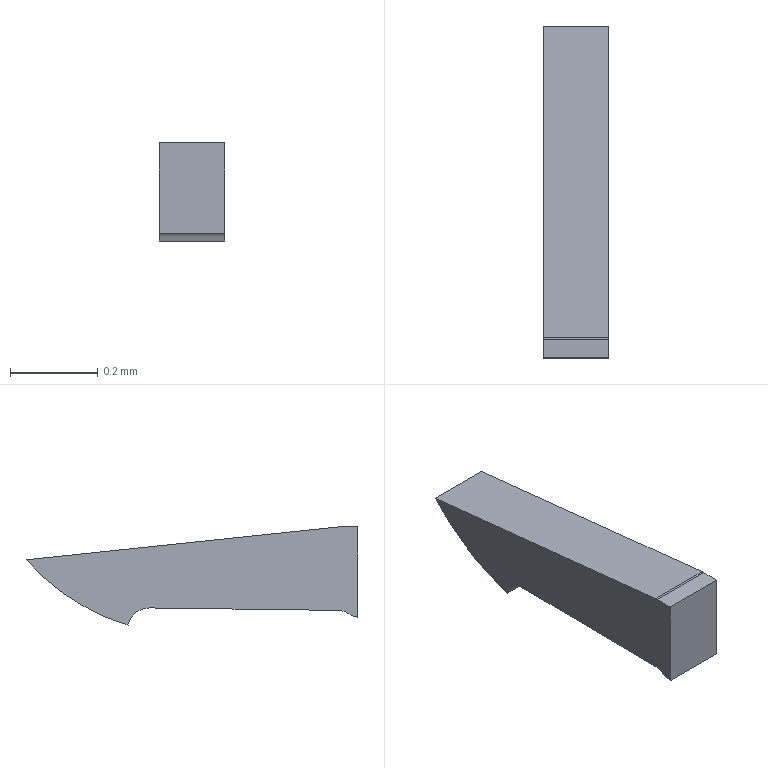Part | Creo | 1 solid | 11 faces | box 0.15 x 0.7581 x 0.2242 mm | volume 0.01667 mm3 | plane 6 | cylinder 5 | commonest cylinder face diameters 0.1 x4 1 x1
STEP:
#1=CARTESIAN_POINT('',(0.,0.,0.));
#2=DIRECTION('',(0.,0.,1.));
#3=DIRECTION('',(1.,0.,0.));
#4=AXIS2_PLACEMENT_3D('',#1,#2,#3);
#5=CARTESIAN_POINT('',(1.21,1.33,-0.16));
#6=VERTEX_POINT('',#5);
#7=CARTESIAN_POINT('',(1.21,1.33,-0.3661));
#8=VERTEX_POINT('',#7);
#9=CARTESIAN_POINT('',(1.21,1.33,-0.16));
#10=DIRECTION('',(0.,0.,-1.));
#11=VECTOR('',#10,0.2061);
#12=LINE('',#9,#11);
#13=EDGE_CURVE('',#6,#8,#12,.T.);
#14=ORIENTED_EDGE('',*,*,#13,.F.);
#15=CARTESIAN_POINT('',(1.21,1.372,-0.16));
#16=VERTEX_POINT('',#15);
#17=CARTESIAN_POINT('',(1.21,1.372,-0.16));
#18=DIRECTION('',(0.,-1.,0.));
#19=VECTOR('',#18,0.04168);
#20=LINE('',#17,#19);
#21=EDGE_CURVE('',#16,#6,#20,.T.);
#22=ORIENTED_EDGE('',*,*,#21,.F.);
#23=CARTESIAN_POINT('',(1.21,1.377,-0.1603));
#24=VERTEX_POINT('',#23);
#25=CARTESIAN_POINT('',(1.21,1.372,-0.21));
#26=DIRECTION('',(-1.,0.,0.));
#27=DIRECTION('',(0.,0.,1.));
#28=AXIS2_PLACEMENT_3D('',#25,#26,#27);
#29=CIRCLE('',#28,0.05);
#30=EDGE_CURVE('',#16,#24,#29,.T.);
#31=ORIENTED_EDGE('',*,*,#30,.T.);
#32=CARTESIAN_POINT('',(1.21,2.088,-0.235));
#33=VERTEX_POINT('',#32);
#34=CARTESIAN_POINT('',(1.21,1.377,-0.1603));
#35=DIRECTION('',(0.,0.9945,-0.1045));
#36=VECTOR('',#35,0.7151);
#37=LINE('',#34,#36);
#38=EDGE_CURVE('',#24,#33,#37,.T.);
#39=ORIENTED_EDGE('',*,*,#38,.T.);
#40=CARTESIAN_POINT('',(1.21,1.855,-0.3842));
#41=VERTEX_POINT('',#40);
#42=CARTESIAN_POINT('',(1.21,1.712,0.09503));
#43=DIRECTION('',(-1.,0.,0.));
#44=DIRECTION('',(0.,0.7512,-0.6601));
#45=AXIS2_PLACEMENT_3D('',#42,#43,#44);
#46=CIRCLE('',#45,0.5);
#47=EDGE_CURVE('',#33,#41,#46,.T.);
#48=ORIENTED_EDGE('',*,*,#47,.T.);
#49=CARTESIAN_POINT('',(1.21,1.806,-0.345));
#50=VERTEX_POINT('',#49);
#51=CARTESIAN_POINT('',(1.21,1.806,-0.395));
#52=DIRECTION('',(1.,0.,0.));
#53=DIRECTION('',(0.,0.9762,0.2167));
#54=AXIS2_PLACEMENT_3D('',#51,#52,#53);
#55=CIRCLE('',#54,0.05);
#56=EDGE_CURVE('',#41,#50,#55,.T.);
#57=ORIENTED_EDGE('',*,*,#56,.T.);
#58=CARTESIAN_POINT('',(1.21,1.377,-0.3506));
#59=VERTEX_POINT('',#58);
#60=CARTESIAN_POINT('',(1.21,1.806,-0.345));
#61=DIRECTION('',(0.,-0.9999,-0.01302));
#62=VECTOR('',#61,0.4289);
#63=LINE('',#60,#62);
#64=EDGE_CURVE('',#50,#59,#63,.T.);
#65=ORIENTED_EDGE('',*,*,#64,.T.);
#66=CARTESIAN_POINT('',(1.21,1.35,-0.3586));
#67=VERTEX_POINT('',#66);
#68=CARTESIAN_POINT('',(1.21,1.378,-0.4006));
#69=DIRECTION('',(1.,0.,0.));
#70=DIRECTION('',(0.,-0.01302,0.9999));
#71=AXIS2_PLACEMENT_3D('',#68,#69,#70);
#72=CIRCLE('',#71,0.05);
#73=EDGE_CURVE('',#59,#67,#72,.T.);
#74=ORIENTED_EDGE('',*,*,#73,.T.);
#75=CARTESIAN_POINT('',(1.21,1.323,-0.3166));
#76=DIRECTION('',(-1.,0.,0.));
#77=DIRECTION('',(0.,0.5423,-0.8402));
#78=AXIS2_PLACEMENT_3D('',#75,#76,#77);
#79=CIRCLE('',#78,0.05);
#80=EDGE_CURVE('',#67,#8,#79,.T.);
#81=ORIENTED_EDGE('',*,*,#80,.T.);
#82=EDGE_LOOP('',(#14,#22,#31,#39,#48,#57,#65,#74,#81));
#83=FACE_OUTER_BOUND('',#82,.F.);
#84=CARTESIAN_POINT('',(1.21,1.709,-0.2721));
#85=DIRECTION('',(1.,0.,0.));
#86=DIRECTION('',(0.,0.,-1.));
#87=AXIS2_PLACEMENT_3D('',#84,#85,#86);
#88=PLANE('',#87);
#89=ADVANCED_FACE('',(#83),#88,.T.);
#90=CARTESIAN_POINT('',(1.06,1.33,-0.16));
#91=VERTEX_POINT('',#90);
#92=CARTESIAN_POINT('',(1.21,1.33,-0.16));
#93=DIRECTION('',(-1.,0.,0.));
#94=VECTOR('',#93,0.15);
#95=LINE('',#92,#94);
#96=EDGE_CURVE('',#6,#91,#95,.T.);
#97=ORIENTED_EDGE('',*,*,#96,.F.);
#98=ORIENTED_EDGE('',*,*,#13,.T.);
#99=CARTESIAN_POINT('',(1.06,1.33,-0.3661));
#100=VERTEX_POINT('',#99);
#101=CARTESIAN_POINT('',(1.06,1.33,-0.3661));
#102=DIRECTION('',(1.,0.,0.));
#103=VECTOR('',#102,0.15);
#104=LINE('',#101,#103);
#105=EDGE_CURVE('',#100,#8,#104,.T.);
#106=ORIENTED_EDGE('',*,*,#105,.F.);
#107=CARTESIAN_POINT('',(1.06,1.33,-0.3661));
#108=DIRECTION('',(0.,0.,1.));
#109=VECTOR('',#108,0.2061);
#110=LINE('',#107,#109);
#111=EDGE_CURVE('',#100,#91,#110,.T.);
#112=ORIENTED_EDGE('',*,*,#111,.T.);
#113=EDGE_LOOP('',(#97,#98,#106,#112));
#114=FACE_OUTER_BOUND('',#113,.F.);
#115=CARTESIAN_POINT('',(1.135,1.33,-0.2631));
#116=DIRECTION('',(0.,1.,0.));
#117=DIRECTION('',(0.,0.,1.));
#118=AXIS2_PLACEMENT_3D('',#115,#116,#117);
#119=PLANE('',#118);
#120=ADVANCED_FACE('',(#114),#119,.F.);
#121=ORIENTED_EDGE('',*,*,#96,.T.);
#122=CARTESIAN_POINT('',(1.06,1.372,-0.16));
#123=VERTEX_POINT('',#122);
#124=CARTESIAN_POINT('',(1.06,1.33,-0.16));
#125=DIRECTION('',(0.,1.,0.));
#126=VECTOR('',#125,0.04168);
#127=LINE('',#124,#126);
#128=EDGE_CURVE('',#91,#123,#127,.T.);
#129=ORIENTED_EDGE('',*,*,#128,.T.);
#130=CARTESIAN_POINT('',(1.21,1.372,-0.16));
#131=DIRECTION('',(-1.,0.,0.));
#132=VECTOR('',#131,0.15);
#133=LINE('',#130,#132);
#134=EDGE_CURVE('',#16,#123,#133,.T.);
#135=ORIENTED_EDGE('',*,*,#134,.F.);
#136=ORIENTED_EDGE('',*,*,#21,.T.);
#137=EDGE_LOOP('',(#121,#129,#135,#136));
#138=FACE_OUTER_BOUND('',#137,.F.);
#139=CARTESIAN_POINT('',(1.135,1.351,-0.16));
#140=DIRECTION('',(0.,0.,1.));
#141=DIRECTION('',(0.,1.,0.));
#142=AXIS2_PLACEMENT_3D('',#139,#140,#141);
#143=PLANE('',#142);
#144=ADVANCED_FACE('',(#138),#143,.T.);
#145=ORIENTED_EDGE('',*,*,#111,.F.);
#146=CARTESIAN_POINT('',(1.06,1.35,-0.3586));
#147=VERTEX_POINT('',#146);
#148=CARTESIAN_POINT('',(1.06,1.323,-0.3166));
#149=DIRECTION('',(1.,0.,0.));
#150=DIRECTION('',(0.,0.1334,-0.9911));
#151=AXIS2_PLACEMENT_3D('',#148,#149,#150);
#152=CIRCLE('',#151,0.05);
#153=EDGE_CURVE('',#100,#147,#152,.T.);
#154=ORIENTED_EDGE('',*,*,#153,.T.);
#155=CARTESIAN_POINT('',(1.06,1.377,-0.3506));
#156=VERTEX_POINT('',#155);
#157=CARTESIAN_POINT('',(1.06,1.378,-0.4006));
#158=DIRECTION('',(-1.,0.,0.));
#159=DIRECTION('',(0.,-0.5423,0.8402));
#160=AXIS2_PLACEMENT_3D('',#157,#158,#159);
#161=CIRCLE('',#160,0.05);
#162=EDGE_CURVE('',#147,#156,#161,.T.);
#163=ORIENTED_EDGE('',*,*,#162,.T.);
#164=CARTESIAN_POINT('',(1.06,1.806,-0.345));
#165=VERTEX_POINT('',#164);
#166=CARTESIAN_POINT('',(1.06,1.377,-0.3506));
#167=DIRECTION('',(0.,0.9999,0.01302));
#168=VECTOR('',#167,0.4289);
#169=LINE('',#166,#168);
#170=EDGE_CURVE('',#156,#165,#169,.T.);
#171=ORIENTED_EDGE('',*,*,#170,.T.);
#172=CARTESIAN_POINT('',(1.06,1.855,-0.3842));
#173=VERTEX_POINT('',#172);
#174=CARTESIAN_POINT('',(1.06,1.806,-0.395));
#175=DIRECTION('',(-1.,0.,0.));
#176=DIRECTION('',(0.,-0.01302,0.9999));
#177=AXIS2_PLACEMENT_3D('',#174,#175,#176);
#178=CIRCLE('',#177,0.05);
#179=EDGE_CURVE('',#165,#173,#178,.T.);
#180=ORIENTED_EDGE('',*,*,#179,.T.);
#181=CARTESIAN_POINT('',(1.06,2.088,-0.235));
#182=VERTEX_POINT('',#181);
#183=CARTESIAN_POINT('',(1.06,1.712,0.09503));
#184=DIRECTION('',(1.,0.,0.));
#185=DIRECTION('',(0.,0.2854,-0.9584));
#186=AXIS2_PLACEMENT_3D('',#183,#184,#185);
#187=CIRCLE('',#186,0.5);
#188=EDGE_CURVE('',#173,#182,#187,.T.);
#189=ORIENTED_EDGE('',*,*,#188,.T.);
#190=CARTESIAN_POINT('',(1.06,1.377,-0.1603));
#191=VERTEX_POINT('',#190);
#192=CARTESIAN_POINT('',(1.06,2.088,-0.235));
#193=DIRECTION('',(0.,-0.9945,0.1045));
#194=VECTOR('',#193,0.7151);
#195=LINE('',#192,#194);
#196=EDGE_CURVE('',#182,#191,#195,.T.);
#197=ORIENTED_EDGE('',*,*,#196,.T.);
#198=CARTESIAN_POINT('',(1.06,1.372,-0.21));
#199=DIRECTION('',(1.,0.,0.));
#200=DIRECTION('',(0.,0.1045,0.9945));
#201=AXIS2_PLACEMENT_3D('',#198,#199,#200);
#202=CIRCLE('',#201,0.05);
#203=EDGE_CURVE('',#191,#123,#202,.T.);
#204=ORIENTED_EDGE('',*,*,#203,.T.);
#205=ORIENTED_EDGE('',*,*,#128,.F.);
#206=EDGE_LOOP('',(#145,#154,#163,#171,#180,#189,#197,#204,#205));
#207=FACE_OUTER_BOUND('',#206,.F.);
#208=CARTESIAN_POINT('',(1.06,1.709,-0.2721));
#209=DIRECTION('',(1.,0.,0.));
#210=DIRECTION('',(0.,0.,-1.));
#211=AXIS2_PLACEMENT_3D('',#208,#209,#210);
#212=PLANE('',#211);
#213=ADVANCED_FACE('',(#207),#212,.F.);
#214=ORIENTED_EDGE('',*,*,#105,.T.);
#215=ORIENTED_EDGE('',*,*,#80,.F.);
#216=CARTESIAN_POINT('',(1.06,1.35,-0.3586));
#217=DIRECTION('',(1.,0.,0.));
#218=VECTOR('',#217,0.15);
#219=LINE('',#216,#218);
#220=EDGE_CURVE('',#147,#67,#219,.T.);
#221=ORIENTED_EDGE('',*,*,#220,.F.);
#222=ORIENTED_EDGE('',*,*,#153,.F.);
#223=EDGE_LOOP('',(#214,#215,#221,#222));
#224=FACE_OUTER_BOUND('',#223,.F.);
#225=CARTESIAN_POINT('',(1.213,1.323,-0.3166));
#226=DIRECTION('',(-1.,0.,0.));
#227=DIRECTION('',(0.,0.5423,-0.8402));
#228=AXIS2_PLACEMENT_3D('',#225,#226,#227);
#229=CYLINDRICAL_SURFACE('',#228,0.05);
#230=ADVANCED_FACE('',(#224),#229,.T.);
#231=ORIENTED_EDGE('',*,*,#162,.F.);
#232=ORIENTED_EDGE('',*,*,#220,.T.);
#233=ORIENTED_EDGE('',*,*,#73,.F.);
#234=CARTESIAN_POINT('',(1.21,1.377,-0.3506));
#235=DIRECTION('',(-1.,0.,0.));
#236=VECTOR('',#235,0.15);
#237=LINE('',#234,#236);
#238=EDGE_CURVE('',#59,#156,#237,.T.);
#239=ORIENTED_EDGE('',*,*,#238,.T.);
#240=EDGE_LOOP('',(#231,#232,#233,#239));
#241=FACE_OUTER_BOUND('',#240,.F.);
#242=CARTESIAN_POINT('',(1.057,1.378,-0.4006));
#243=DIRECTION('',(1.,0.,0.));
#244=DIRECTION('',(0.,-0.01302,0.9999));
#245=AXIS2_PLACEMENT_3D('',#242,#243,#244);
#246=CYLINDRICAL_SURFACE('',#245,0.05);
#247=ADVANCED_FACE('',(#241),#246,.F.);
#248=ORIENTED_EDGE('',*,*,#170,.F.);
#249=ORIENTED_EDGE('',*,*,#238,.F.);
#250=ORIENTED_EDGE('',*,*,#64,.F.);
#251=CARTESIAN_POINT('',(1.06,1.806,-0.345));
#252=DIRECTION('',(1.,0.,0.));
#253=VECTOR('',#252,0.15);
#254=LINE('',#251,#253);
#255=EDGE_CURVE('',#165,#50,#254,.T.);
#256=ORIENTED_EDGE('',*,*,#255,.F.);
#257=EDGE_LOOP('',(#248,#249,#250,#256));
#258=FACE_OUTER_BOUND('',#257,.F.);
#259=CARTESIAN_POINT('',(1.135,1.591,-0.3478));
#260=DIRECTION('',(0.,-0.01302,0.9999));
#261=DIRECTION('',(0.,-0.9999,-0.01302));
#262=AXIS2_PLACEMENT_3D('',#259,#260,#261);
#263=PLANE('',#262);
#264=ADVANCED_FACE('',(#258),#263,.F.);
#265=ORIENTED_EDGE('',*,*,#179,.F.);
#266=ORIENTED_EDGE('',*,*,#255,.T.);
#267=ORIENTED_EDGE('',*,*,#56,.F.);
#268=CARTESIAN_POINT('',(1.21,1.855,-0.3842));
#269=DIRECTION('',(-1.,0.,0.));
#270=VECTOR('',#269,0.15);
#271=LINE('',#268,#270);
#272=EDGE_CURVE('',#41,#173,#271,.T.);
#273=ORIENTED_EDGE('',*,*,#272,.T.);
#274=EDGE_LOOP('',(#265,#266,#267,#273));
#275=FACE_OUTER_BOUND('',#274,.F.);
#276=CARTESIAN_POINT('',(1.057,1.806,-0.395));
#277=DIRECTION('',(1.,0.,0.));
#278=DIRECTION('',(0.,0.9762,0.2167));
#279=AXIS2_PLACEMENT_3D('',#276,#277,#278);
#280=CYLINDRICAL_SURFACE('',#279,0.05);
#281=ADVANCED_FACE('',(#275),#280,.F.);
#282=ORIENTED_EDGE('',*,*,#188,.F.);
#283=ORIENTED_EDGE('',*,*,#272,.F.);
#284=ORIENTED_EDGE('',*,*,#47,.F.);
#285=CARTESIAN_POINT('',(1.21,2.088,-0.235));
#286=DIRECTION('',(-1.,0.,0.));
#287=VECTOR('',#286,0.15);
#288=LINE('',#285,#287);
#289=EDGE_CURVE('',#33,#182,#288,.T.);
#290=ORIENTED_EDGE('',*,*,#289,.T.);
#291=EDGE_LOOP('',(#282,#283,#284,#290));
#292=FACE_OUTER_BOUND('',#291,.F.);
#293=CARTESIAN_POINT('',(1.213,1.712,0.09503));
#294=DIRECTION('',(-1.,0.,0.));
#295=DIRECTION('',(0.,0.7512,-0.6601));
#296=AXIS2_PLACEMENT_3D('',#293,#294,#295);
#297=CYLINDRICAL_SURFACE('',#296,0.5);
#298=ADVANCED_FACE('',(#292),#297,.T.);
#299=ORIENTED_EDGE('',*,*,#196,.F.);
#300=ORIENTED_EDGE('',*,*,#289,.F.);
#301=ORIENTED_EDGE('',*,*,#38,.F.);
#302=CARTESIAN_POINT('',(1.06,1.377,-0.1603));
#303=DIRECTION('',(1.,0.,0.));
#304=VECTOR('',#303,0.15);
#305=LINE('',#302,#304);
#306=EDGE_CURVE('',#191,#24,#305,.T.);
#307=ORIENTED_EDGE('',*,*,#306,.F.);
#308=EDGE_LOOP('',(#299,#300,#301,#307));
#309=FACE_OUTER_BOUND('',#308,.F.);
#310=CARTESIAN_POINT('',(1.135,1.732,-0.1976));
#311=DIRECTION('',(0.,0.1045,0.9945));
#312=DIRECTION('',(0.,0.9945,-0.1045));
#313=AXIS2_PLACEMENT_3D('',#310,#311,#312);
#314=PLANE('',#313);
#315=ADVANCED_FACE('',(#309),#314,.T.);
#316=ORIENTED_EDGE('',*,*,#203,.F.);
#317=ORIENTED_EDGE('',*,*,#306,.T.);
#318=ORIENTED_EDGE('',*,*,#30,.F.);
#319=ORIENTED_EDGE('',*,*,#134,.T.);
#320=EDGE_LOOP('',(#316,#317,#318,#319));
#321=FACE_OUTER_BOUND('',#320,.F.);
#322=CARTESIAN_POINT('',(1.213,1.372,-0.21));
#323=DIRECTION('',(-1.,0.,0.));
#324=DIRECTION('',(0.,0.,1.));
#325=AXIS2_PLACEMENT_3D('',#322,#323,#324);
#326=CYLINDRICAL_SURFACE('',#325,0.05);
#327=ADVANCED_FACE('',(#321),#326,.T.);
#328=CLOSED_SHELL('',(#89,#120,#144,#213,#230,#247,#264,#281,#298,#315,#327));
#329=MANIFOLD_SOLID_BREP('',#328);
#330=(LENGTH_UNIT()NAMED_UNIT(*)SI_UNIT(.MILLI.,.METRE.));
#331=UNCERTAINTY_MEASURE_WITH_UNIT(LENGTH_MEASURE(0.00008046),#330,'','');
#332=(NAMED_UNIT(*)PLANE_ANGLE_UNIT()SI_UNIT($,.RADIAN.));
#333=PLANE_ANGLE_MEASURE_WITH_UNIT(PLANE_ANGLE_MEASURE(0.01745),#332);
#334=(CONVERSION_BASED_UNIT('DEGREE',#333)NAMED_UNIT(*)PLANE_ANGLE_UNIT());
#335=(NAMED_UNIT(*)SI_UNIT($,.STERADIAN.)SOLID_ANGLE_UNIT());
#336=(GEOMETRIC_REPRESENTATION_CONTEXT(3)GLOBAL_UNCERTAINTY_ASSIGNED_CONTEXT((#331))GLOBAL_UNIT_ASSIGNED_CONTEXT((#330,#334,#335))REPRESENTATION_CONTEXT('',''));
#337=ADVANCED_BREP_SHAPE_REPRESENTATION('',(#4,#329),#336);